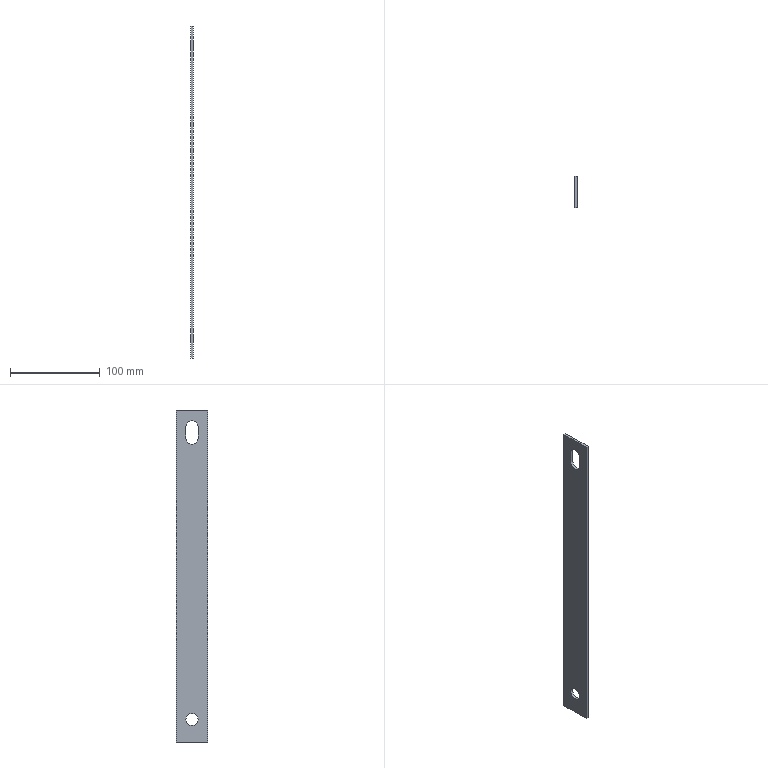Part | NX | features solid 2 | 1 solid | 11 faces | box 3 x 35 x 370 mm | volume 37485 mm3 | plane 8 | cylinder 3 | commonest cylinder face diameters 13.5 x3
STEP:
#1=CARTESIAN_POINT('',(1010.,-333.25,136.25));
#2=VERTEX_POINT('',#1);
#3=CARTESIAN_POINT('',(1010.,-346.75,136.25));
#4=VERTEX_POINT('',#3);
#5=CARTESIAN_POINT('',(1010.,-340.,136.25));
#6=DIRECTION('',(1.,0.,0.));
#7=DIRECTION('',(0.,1.,0.));
#8=AXIS2_PLACEMENT_3D('',#5,#6,#7);
#9=CIRCLE('',#8,6.75);
#10=EDGE_CURVE('',#2,#4,#9,.T.);
#11=ORIENTED_EDGE('',*,*,#10,.F.);
#12=CARTESIAN_POINT('',(1013.,-333.25,136.25));
#13=VERTEX_POINT('',#12);
#14=CARTESIAN_POINT('',(1013.,-333.25,136.25));
#15=DIRECTION('',(-1.,0.,0.));
#16=VECTOR('',#15,1000.);
#17=LINE('',#14,#16);
#18=EDGE_CURVE('',#13,#2,#17,.T.);
#19=ORIENTED_EDGE('',*,*,#18,.F.);
#20=CARTESIAN_POINT('',(1013.,-346.75,136.25));
#21=VERTEX_POINT('',#20);
#22=CARTESIAN_POINT('',(1013.,-340.,136.25));
#23=DIRECTION('',(1.,0.,0.));
#24=DIRECTION('',(0.,1.,0.));
#25=AXIS2_PLACEMENT_3D('',#22,#23,#24);
#26=CIRCLE('',#25,6.75);
#27=EDGE_CURVE('',#13,#21,#26,.T.);
#28=ORIENTED_EDGE('',*,*,#27,.T.);
#29=CARTESIAN_POINT('',(1013.,-346.75,136.25));
#30=DIRECTION('',(-1.,0.,0.));
#31=VECTOR('',#30,1000.);
#32=LINE('',#29,#31);
#33=EDGE_CURVE('',#21,#4,#32,.T.);
#34=ORIENTED_EDGE('',*,*,#33,.T.);
#35=EDGE_LOOP('',(#11,#19,#28,#34));
#36=FACE_BOUND('',#35,.T.);
#37=CARTESIAN_POINT('',(1013.,-340.,136.25));
#38=DIRECTION('',(-1.,0.,0.));
#39=DIRECTION('',(0.,1.,0.));
#40=AXIS2_PLACEMENT_3D('',#37,#38,#39);
#41=CYLINDRICAL_SURFACE('',#40,6.75);
#42=ADVANCED_FACE('',(#36),#41,.F.);
#43=CARTESIAN_POINT('',(1010.,-333.25,123.75));
#44=VERTEX_POINT('',#43);
#45=CARTESIAN_POINT('',(1010.,-333.25,136.25));
#46=DIRECTION('',(0.,0.,-1.));
#47=VECTOR('',#46,1000.);
#48=LINE('',#45,#47);
#49=EDGE_CURVE('',#2,#44,#48,.T.);
#50=ORIENTED_EDGE('',*,*,#49,.T.);
#51=CARTESIAN_POINT('',(1013.,-333.25,123.75));
#52=VERTEX_POINT('',#51);
#53=CARTESIAN_POINT('',(1013.,-333.25,123.75));
#54=DIRECTION('',(-1.,0.,0.));
#55=VECTOR('',#54,1000.);
#56=LINE('',#53,#55);
#57=EDGE_CURVE('',#52,#44,#56,.T.);
#58=ORIENTED_EDGE('',*,*,#57,.F.);
#59=CARTESIAN_POINT('',(1013.,-333.25,136.25));
#60=DIRECTION('',(0.,0.,-1.));
#61=VECTOR('',#60,1000.);
#62=LINE('',#59,#61);
#63=EDGE_CURVE('',#13,#52,#62,.T.);
#64=ORIENTED_EDGE('',*,*,#63,.F.);
#65=ORIENTED_EDGE('',*,*,#18,.T.);
#66=EDGE_LOOP('',(#50,#58,#64,#65));
#67=FACE_BOUND('',#66,.T.);
#68=CARTESIAN_POINT('',(1013.,-333.25,136.25));
#69=DIRECTION('',(0.,-1.,0.));
#70=DIRECTION('',(-1.,0.,0.));
#71=AXIS2_PLACEMENT_3D('',#68,#69,#70);
#72=PLANE('',#71);
#73=ADVANCED_FACE('',(#67),#72,.T.);
#74=CARTESIAN_POINT('',(1010.,-346.75,123.75));
#75=VERTEX_POINT('',#74);
#76=CARTESIAN_POINT('',(1010.,-340.,123.75));
#77=DIRECTION('',(1.,0.,0.));
#78=DIRECTION('',(0.,1.,0.));
#79=AXIS2_PLACEMENT_3D('',#76,#77,#78);
#80=CIRCLE('',#79,6.75);
#81=EDGE_CURVE('',#75,#44,#80,.T.);
#82=ORIENTED_EDGE('',*,*,#81,.F.);
#83=CARTESIAN_POINT('',(1013.,-346.75,123.75));
#84=VERTEX_POINT('',#83);
#85=CARTESIAN_POINT('',(1013.,-346.75,123.75));
#86=DIRECTION('',(-1.,0.,0.));
#87=VECTOR('',#86,1000.);
#88=LINE('',#85,#87);
#89=EDGE_CURVE('',#84,#75,#88,.T.);
#90=ORIENTED_EDGE('',*,*,#89,.F.);
#91=CARTESIAN_POINT('',(1013.,-340.,123.75));
#92=DIRECTION('',(1.,0.,0.));
#93=DIRECTION('',(0.,1.,0.));
#94=AXIS2_PLACEMENT_3D('',#91,#92,#93);
#95=CIRCLE('',#94,6.75);
#96=EDGE_CURVE('',#84,#52,#95,.T.);
#97=ORIENTED_EDGE('',*,*,#96,.T.);
#98=ORIENTED_EDGE('',*,*,#57,.T.);
#99=EDGE_LOOP('',(#82,#90,#97,#98));
#100=FACE_BOUND('',#99,.T.);
#101=CARTESIAN_POINT('',(1013.,-340.,123.75));
#102=DIRECTION('',(-1.,0.,0.));
#103=DIRECTION('',(0.,1.,0.));
#104=AXIS2_PLACEMENT_3D('',#101,#102,#103);
#105=CYLINDRICAL_SURFACE('',#104,6.75);
#106=ADVANCED_FACE('',(#100),#105,.F.);
#107=CARTESIAN_POINT('',(1010.,-322.5,-215.));
#108=VERTEX_POINT('',#107);
#109=CARTESIAN_POINT('',(1010.,-322.5,155.));
#110=VERTEX_POINT('',#109);
#111=CARTESIAN_POINT('',(1010.,-322.5,-215.));
#112=DIRECTION('',(0.,0.,1.));
#113=VECTOR('',#112,1000.);
#114=LINE('',#111,#113);
#115=EDGE_CURVE('',#108,#110,#114,.T.);
#116=ORIENTED_EDGE('',*,*,#115,.T.);
#117=CARTESIAN_POINT('',(1013.,-322.5,155.));
#118=VERTEX_POINT('',#117);
#119=CARTESIAN_POINT('',(1013.,-322.5,155.));
#120=DIRECTION('',(-1.,0.,0.));
#121=VECTOR('',#120,1000.);
#122=LINE('',#119,#121);
#123=EDGE_CURVE('',#118,#110,#122,.T.);
#124=ORIENTED_EDGE('',*,*,#123,.F.);
#125=CARTESIAN_POINT('',(1013.,-322.5,-215.));
#126=VERTEX_POINT('',#125);
#127=CARTESIAN_POINT('',(1013.,-322.5,-215.));
#128=DIRECTION('',(0.,0.,1.));
#129=VECTOR('',#128,1000.);
#130=LINE('',#127,#129);
#131=EDGE_CURVE('',#126,#118,#130,.T.);
#132=ORIENTED_EDGE('',*,*,#131,.F.);
#133=CARTESIAN_POINT('',(1013.,-322.5,-215.));
#134=DIRECTION('',(-1.,0.,0.));
#135=VECTOR('',#134,1000.);
#136=LINE('',#133,#135);
#137=EDGE_CURVE('',#126,#108,#136,.T.);
#138=ORIENTED_EDGE('',*,*,#137,.T.);
#139=EDGE_LOOP('',(#116,#124,#132,#138));
#140=FACE_BOUND('',#139,.T.);
#141=CARTESIAN_POINT('',(1013.,-322.5,-215.));
#142=DIRECTION('',(0.,1.,0.));
#143=DIRECTION('',(0.,0.,1.));
#144=AXIS2_PLACEMENT_3D('',#141,#142,#143);
#145=PLANE('',#144);
#146=ADVANCED_FACE('',(#140),#145,.T.);
#147=CARTESIAN_POINT('',(1010.,-357.5,155.));
#148=VERTEX_POINT('',#147);
#149=CARTESIAN_POINT('',(1010.,-322.5,155.));
#150=DIRECTION('',(0.,-1.,0.));
#151=VECTOR('',#150,1000.);
#152=LINE('',#149,#151);
#153=EDGE_CURVE('',#110,#148,#152,.T.);
#154=ORIENTED_EDGE('',*,*,#153,.T.);
#155=CARTESIAN_POINT('',(1013.,-357.5,155.));
#156=VERTEX_POINT('',#155);
#157=CARTESIAN_POINT('',(1013.,-357.5,155.));
#158=DIRECTION('',(-1.,0.,0.));
#159=VECTOR('',#158,1000.);
#160=LINE('',#157,#159);
#161=EDGE_CURVE('',#156,#148,#160,.T.);
#162=ORIENTED_EDGE('',*,*,#161,.F.);
#163=CARTESIAN_POINT('',(1013.,-322.5,155.));
#164=DIRECTION('',(0.,-1.,0.));
#165=VECTOR('',#164,1000.);
#166=LINE('',#163,#165);
#167=EDGE_CURVE('',#118,#156,#166,.T.);
#168=ORIENTED_EDGE('',*,*,#167,.F.);
#169=ORIENTED_EDGE('',*,*,#123,.T.);
#170=EDGE_LOOP('',(#154,#162,#168,#169));
#171=FACE_BOUND('',#170,.T.);
#172=CARTESIAN_POINT('',(1013.,-322.5,155.));
#173=DIRECTION('',(0.,0.,1.));
#174=DIRECTION('',(-1.,0.,0.));
#175=AXIS2_PLACEMENT_3D('',#172,#173,#174);
#176=PLANE('',#175);
#177=ADVANCED_FACE('',(#171),#176,.T.);
#178=CARTESIAN_POINT('',(1010.,-357.5,-215.));
#179=VERTEX_POINT('',#178);
#180=CARTESIAN_POINT('',(1010.,-357.5,85.));
#181=DIRECTION('',(0.,0.,-1.));
#182=VECTOR('',#181,1000.);
#183=LINE('',#180,#182);
#184=EDGE_CURVE('',#148,#179,#183,.T.);
#185=ORIENTED_EDGE('',*,*,#184,.T.);
#186=CARTESIAN_POINT('',(1013.,-357.5,-215.));
#187=VERTEX_POINT('',#186);
#188=CARTESIAN_POINT('',(1013.,-357.5,-215.));
#189=DIRECTION('',(-1.,0.,0.));
#190=VECTOR('',#189,1000.);
#191=LINE('',#188,#190);
#192=EDGE_CURVE('',#187,#179,#191,.T.);
#193=ORIENTED_EDGE('',*,*,#192,.F.);
#194=CARTESIAN_POINT('',(1013.,-357.5,85.));
#195=DIRECTION('',(0.,0.,-1.));
#196=VECTOR('',#195,1000.);
#197=LINE('',#194,#196);
#198=EDGE_CURVE('',#156,#187,#197,.T.);
#199=ORIENTED_EDGE('',*,*,#198,.F.);
#200=ORIENTED_EDGE('',*,*,#161,.T.);
#201=EDGE_LOOP('',(#185,#193,#199,#200));
#202=FACE_BOUND('',#201,.T.);
#203=CARTESIAN_POINT('',(1013.,-357.5,85.));
#204=DIRECTION('',(0.,-1.,0.));
#205=DIRECTION('',(0.,0.,-1.));
#206=AXIS2_PLACEMENT_3D('',#203,#204,#205);
#207=PLANE('',#206);
#208=ADVANCED_FACE('',(#202),#207,.T.);
#209=CARTESIAN_POINT('',(1013.,-333.25,-190.));
#210=VERTEX_POINT('',#209);
#211=CARTESIAN_POINT('',(1013.,-340.,-190.));
#212=DIRECTION('',(1.,0.,0.));
#213=DIRECTION('',(0.,1.,0.));
#214=AXIS2_PLACEMENT_3D('',#211,#212,#213);
#215=CIRCLE('',#214,6.75);
#216=EDGE_CURVE('',#210,#210,#215,.T.);
#217=ORIENTED_EDGE('',*,*,#216,.T.);
#218=EDGE_LOOP('',(#217));
#219=FACE_BOUND('',#218,.T.);
#220=CARTESIAN_POINT('',(1010.,-333.25,-190.));
#221=VERTEX_POINT('',#220);
#222=CARTESIAN_POINT('',(1010.,-340.,-190.));
#223=DIRECTION('',(1.,0.,0.));
#224=DIRECTION('',(0.,1.,0.));
#225=AXIS2_PLACEMENT_3D('',#222,#223,#224);
#226=CIRCLE('',#225,6.75);
#227=EDGE_CURVE('',#221,#221,#226,.T.);
#228=ORIENTED_EDGE('',*,*,#227,.F.);
#229=EDGE_LOOP('',(#228));
#230=FACE_BOUND('',#229,.T.);
#231=CARTESIAN_POINT('',(1013.,-340.,-190.));
#232=DIRECTION('',(-1.,0.,0.));
#233=DIRECTION('',(0.,1.,0.));
#234=AXIS2_PLACEMENT_3D('',#231,#232,#233);
#235=CYLINDRICAL_SURFACE('',#234,6.75);
#236=ADVANCED_FACE('',(#219,#230),#235,.F.);
#237=CARTESIAN_POINT('',(1010.,-357.5,-215.));
#238=DIRECTION('',(0.,1.,0.));
#239=VECTOR('',#238,1000.);
#240=LINE('',#237,#239);
#241=EDGE_CURVE('',#179,#108,#240,.T.);
#242=ORIENTED_EDGE('',*,*,#241,.T.);
#243=ORIENTED_EDGE('',*,*,#137,.F.);
#244=CARTESIAN_POINT('',(1013.,-357.5,-215.));
#245=DIRECTION('',(0.,1.,0.));
#246=VECTOR('',#245,1000.);
#247=LINE('',#244,#246);
#248=EDGE_CURVE('',#187,#126,#247,.T.);
#249=ORIENTED_EDGE('',*,*,#248,.F.);
#250=ORIENTED_EDGE('',*,*,#192,.T.);
#251=EDGE_LOOP('',(#242,#243,#249,#250));
#252=FACE_BOUND('',#251,.T.);
#253=CARTESIAN_POINT('',(1013.,-357.5,-215.));
#254=DIRECTION('',(0.,0.,-1.));
#255=DIRECTION('',(1.,0.,0.));
#256=AXIS2_PLACEMENT_3D('',#253,#254,#255);
#257=PLANE('',#256);
#258=ADVANCED_FACE('',(#252),#257,.T.);
#259=CARTESIAN_POINT('',(1010.,-346.75,123.75));
#260=DIRECTION('',(0.,0.,1.));
#261=VECTOR('',#260,1000.);
#262=LINE('',#259,#261);
#263=EDGE_CURVE('',#75,#4,#262,.T.);
#264=ORIENTED_EDGE('',*,*,#263,.T.);
#265=ORIENTED_EDGE('',*,*,#33,.F.);
#266=CARTESIAN_POINT('',(1013.,-346.75,123.75));
#267=DIRECTION('',(0.,0.,1.));
#268=VECTOR('',#267,1000.);
#269=LINE('',#266,#268);
#270=EDGE_CURVE('',#84,#21,#269,.T.);
#271=ORIENTED_EDGE('',*,*,#270,.F.);
#272=ORIENTED_EDGE('',*,*,#89,.T.);
#273=EDGE_LOOP('',(#264,#265,#271,#272));
#274=FACE_BOUND('',#273,.T.);
#275=CARTESIAN_POINT('',(1013.,-346.75,123.75));
#276=DIRECTION('',(0.,1.,0.));
#277=DIRECTION('',(1.,0.,0.));
#278=AXIS2_PLACEMENT_3D('',#275,#276,#277);
#279=PLANE('',#278);
#280=ADVANCED_FACE('',(#274),#279,.T.);
#281=ORIENTED_EDGE('',*,*,#131,.T.);
#282=ORIENTED_EDGE('',*,*,#167,.T.);
#283=ORIENTED_EDGE('',*,*,#198,.T.);
#284=ORIENTED_EDGE('',*,*,#248,.T.);
#285=EDGE_LOOP('',(#281,#282,#283,#284));
#286=FACE_BOUND('',#285,.T.);
#287=ORIENTED_EDGE('',*,*,#216,.F.);
#288=EDGE_LOOP('',(#287));
#289=FACE_BOUND('',#288,.T.);
#290=ORIENTED_EDGE('',*,*,#27,.F.);
#291=ORIENTED_EDGE('',*,*,#63,.T.);
#292=ORIENTED_EDGE('',*,*,#96,.F.);
#293=ORIENTED_EDGE('',*,*,#270,.T.);
#294=EDGE_LOOP('',(#290,#291,#292,#293));
#295=FACE_BOUND('',#294,.T.);
#296=CARTESIAN_POINT('',(1013.,-322.5,85.));
#297=DIRECTION('',(-1.,0.,0.));
#298=DIRECTION('',(0.,1.,0.));
#299=AXIS2_PLACEMENT_3D('',#296,#297,#298);
#300=PLANE('',#299);
#301=ADVANCED_FACE('',(#286,#289,#295),#300,.F.);
#302=ORIENTED_EDGE('',*,*,#115,.F.);
#303=ORIENTED_EDGE('',*,*,#241,.F.);
#304=ORIENTED_EDGE('',*,*,#184,.F.);
#305=ORIENTED_EDGE('',*,*,#153,.F.);
#306=EDGE_LOOP('',(#302,#303,#304,#305));
#307=FACE_BOUND('',#306,.T.);
#308=ORIENTED_EDGE('',*,*,#227,.T.);
#309=EDGE_LOOP('',(#308));
#310=FACE_BOUND('',#309,.T.);
#311=ORIENTED_EDGE('',*,*,#10,.T.);
#312=ORIENTED_EDGE('',*,*,#263,.F.);
#313=ORIENTED_EDGE('',*,*,#81,.T.);
#314=ORIENTED_EDGE('',*,*,#49,.F.);
#315=EDGE_LOOP('',(#311,#312,#313,#314));
#316=FACE_BOUND('',#315,.T.);
#317=CARTESIAN_POINT('',(1010.,-322.5,85.));
#318=DIRECTION('',(-1.,0.,0.));
#319=DIRECTION('',(0.,1.,0.));
#320=AXIS2_PLACEMENT_3D('',#317,#318,#319);
#321=PLANE('',#320);
#322=ADVANCED_FACE('',(#307,#310,#316),#321,.T.);
#323=CLOSED_SHELL('',(#42,#73,#106,#146,#177,#208,#236,#258,#280,#301,#322));
#324=MANIFOLD_SOLID_BREP('',#323);
#325=(LENGTH_UNIT()NAMED_UNIT(*)SI_UNIT(.MILLI.,.METRE.));
#326=UNCERTAINTY_MEASURE_WITH_UNIT(LENGTH_MEASURE(0.00001),#325,'','');
#327=(NAMED_UNIT(*)PLANE_ANGLE_UNIT()SI_UNIT($,.RADIAN.));
#328=(NAMED_UNIT(*)SI_UNIT($,.STERADIAN.)SOLID_ANGLE_UNIT());
#329=(GEOMETRIC_REPRESENTATION_CONTEXT(3)GLOBAL_UNCERTAINTY_ASSIGNED_CONTEXT((#326))GLOBAL_UNIT_ASSIGNED_CONTEXT((#325,#327,#328))REPRESENTATION_CONTEXT('',''));
#330=ADVANCED_BREP_SHAPE_REPRESENTATION('',(#324),#329);